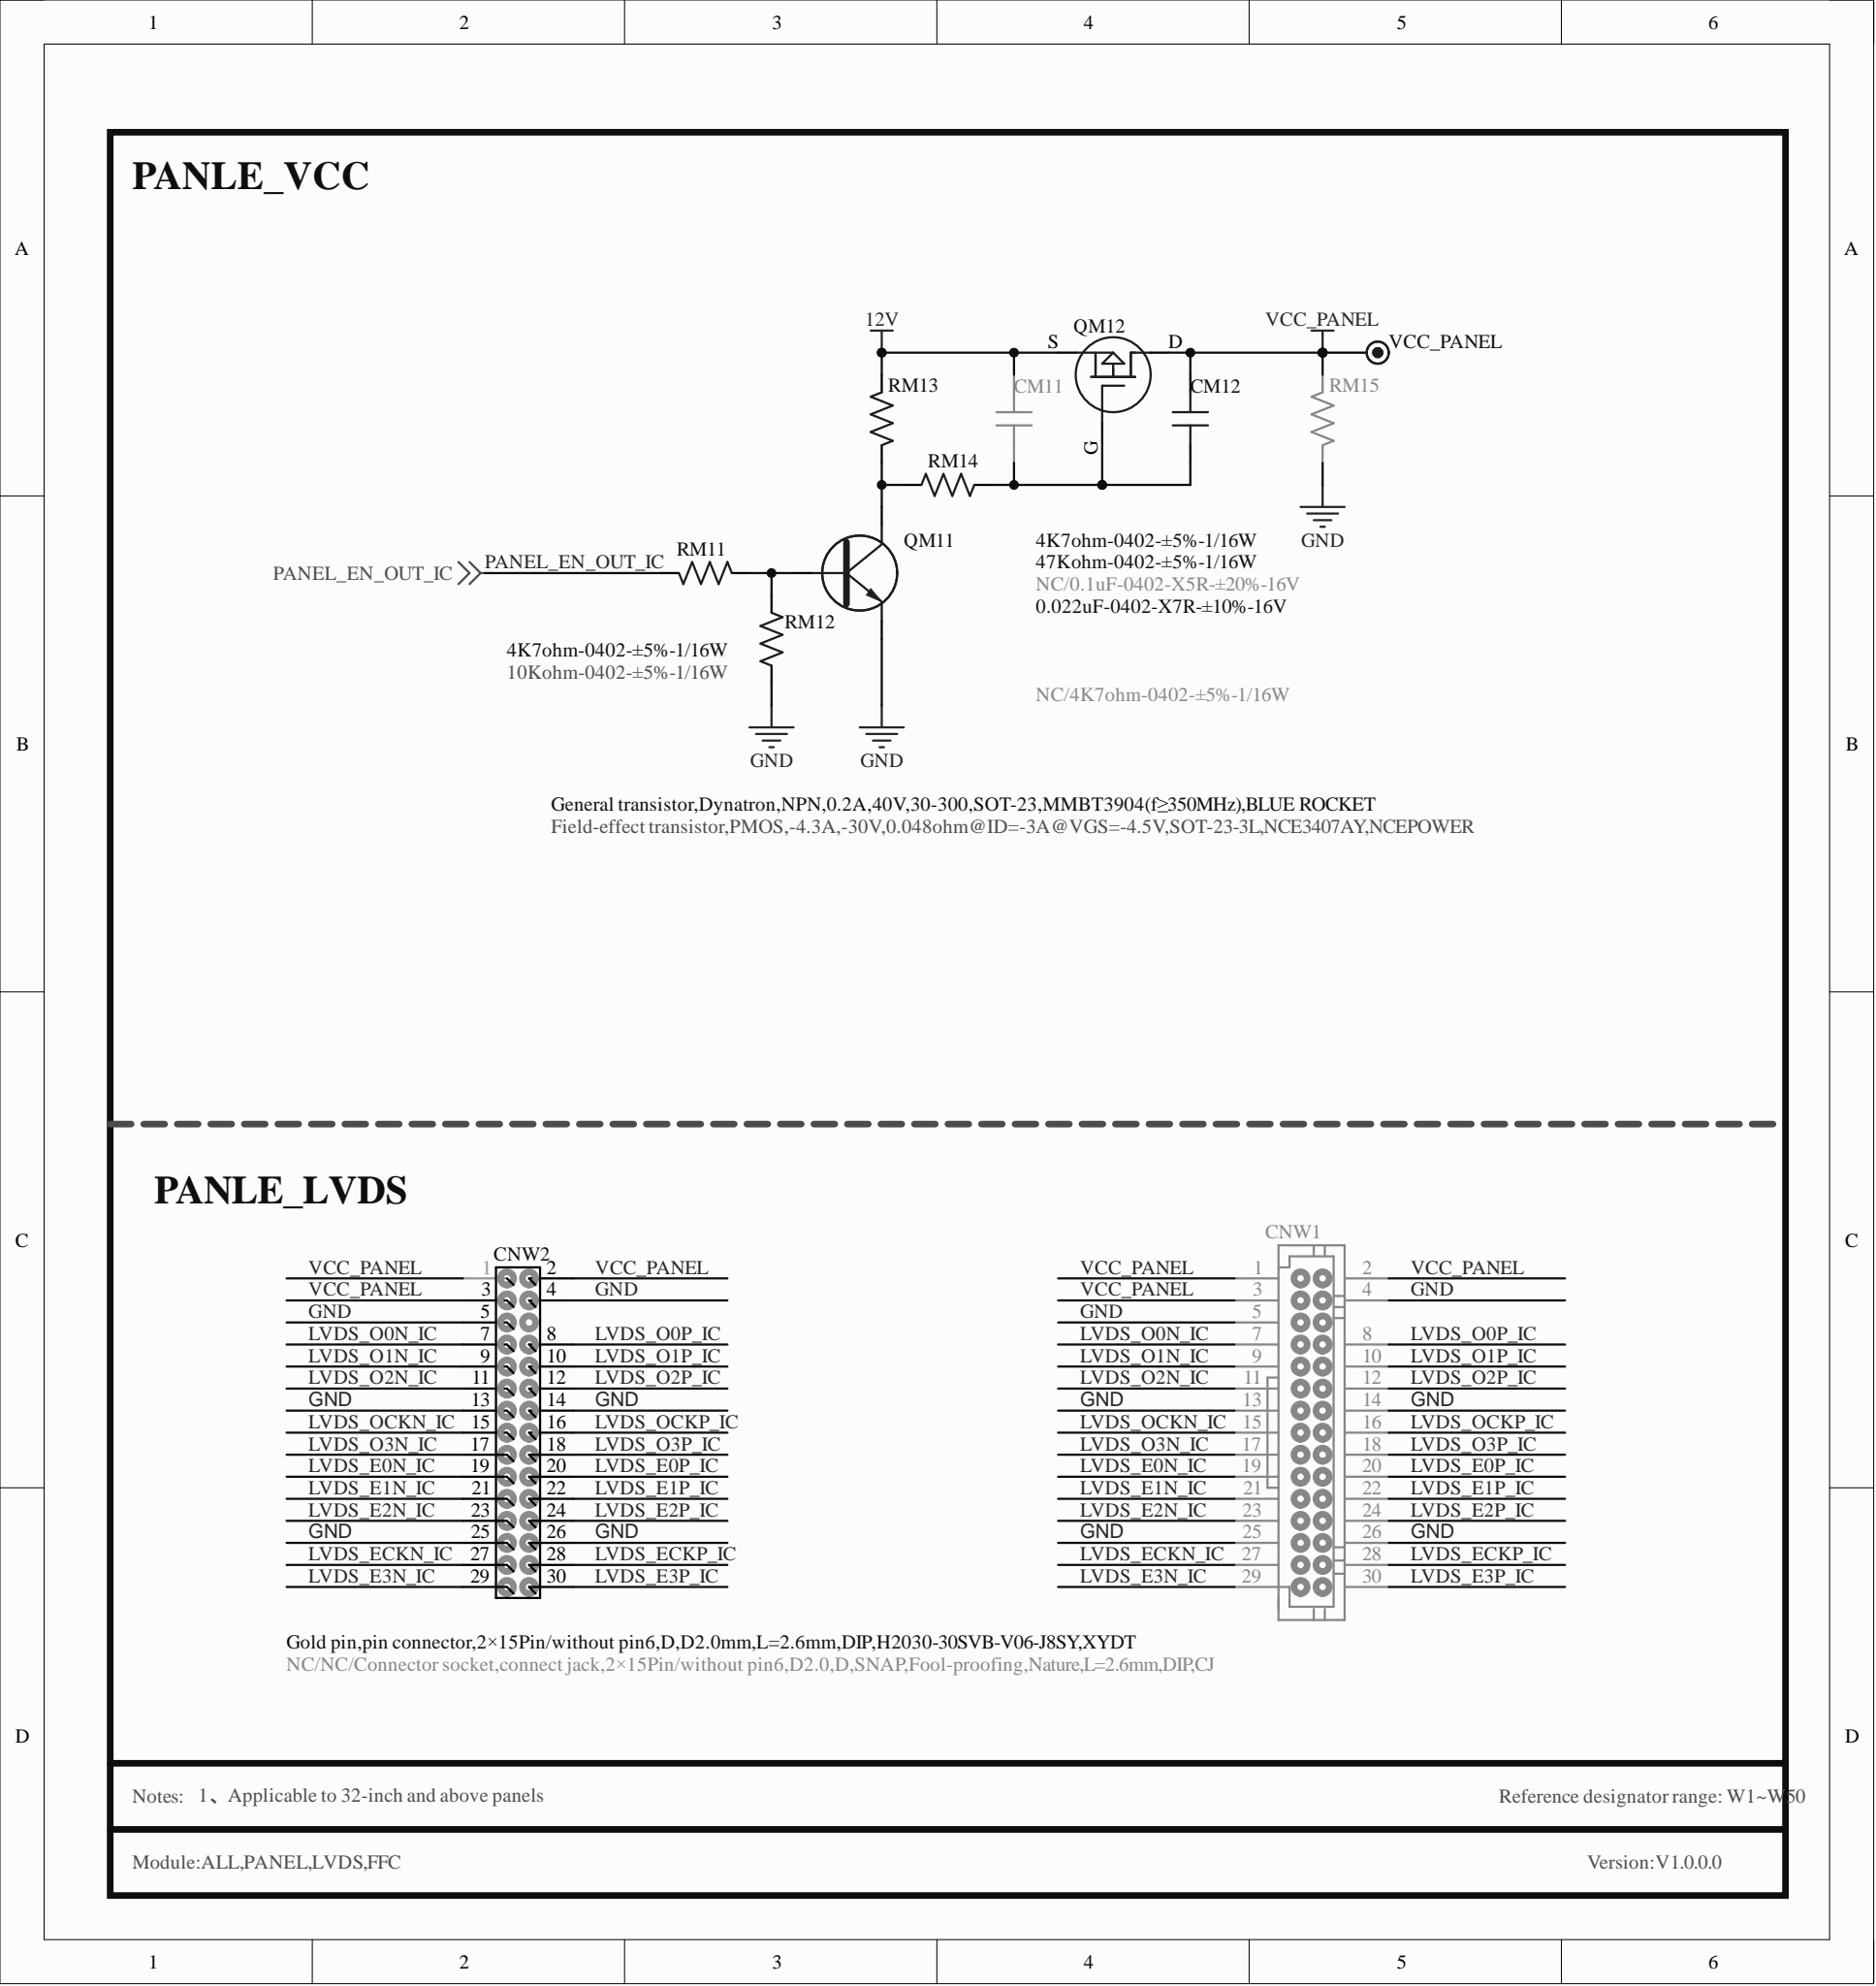Circuit board | Altium Designer | 578 parts | 300 nets | one sheet of the schematic
Parts on this sheet (reference | value | footprint):
CM11 | NC/0.1uF-0402-X5R-±20%-16V | C0402
CM12 | 0.022uF-0402-X7R-±10%-16V | C0402
CNW1 | NC/NC/Connector socket,connect jack,2×15Pin/without pin6,D2.0,D,SNAP,Fool-proofing,Nature,L=2.6mm,DIP,CJ | SIP2*15/2.0D-11
CNW2 | Gold pin,pin connector,2×15Pin/without pin6,D,D2.0mm,L=2.6mm,DIP,H2030-30SVB-V06-J8SY,XYDT | SIP2*15/2.0D-2
QM11 | General transistor,Dynatron,NPN,0.2A,40V,30-300,SOT-23,MMBT3904(f=350MHz),BLUE ROCKET | SOT-23
QM12 | Field-effect transistor,PMOS,-4.3A,-30V,0.048ohm@ID=-3A@VGS=-4.5V,SOT-23-3L,NCE3407AY,NCEPOWER | SOT-23-1
RM11 | 4K7ohm-0402-±5%-1/16W | R0402
RM12 | 10Kohm-0402-±5%-1/16W | R0402
RM13 | 4K7ohm-0402-±5%-1/16W | R0402
RM14 | 47Kohm-0402-±5%-1/16W | R0402
RM15 | NC/4K7ohm-0402-±5%-1/16W | R0402
VCC_PANEL | TEST | TP
Nets of these parts (net: part-pin ...):
VCC_PANEL: CM12-1 QM12-D RM15-1 VCC_PANEL-1 CNW1-1 CNW1-2 CNW1-3 CNW2-1 CNW2-2 CNW2-3
PANEL_EN_OUT_IC: RM11-1
NetQM11_C: QM11-C RM13-2 RM14-1
NetQM11_B: QM11-B RM11-2 RM12-1
NetCM11_1: CM11-1 CM12-2 QM12-G RM14-2
LVDS_OCKP_IC: CNW1-16 CNW2-16
LVDS_OCKN_IC: CNW1-15 CNW2-15
LVDS_O3P_IC: CNW1-18 CNW2-18
LVDS_O3N_IC: CNW1-17 CNW2-17
LVDS_O2P_IC: CNW1-12 CNW2-12
LVDS_O2N_IC: CNW1-11 CNW2-11
LVDS_O1P_IC: CNW1-10 CNW2-10
LVDS_O1N_IC: CNW1-9 CNW2-9
LVDS_O0P_IC: CNW1-8 CNW2-8
LVDS_O0N_IC: CNW1-7 CNW2-7
LVDS_ECKP_IC: CNW1-28 CNW2-28
LVDS_ECKN_IC: CNW1-27 CNW2-27
LVDS_E3P_IC: CNW1-30 CNW2-30
LVDS_E3N_IC: CNW1-29 CNW2-29
LVDS_E2P_IC: CNW1-24 CNW2-24
LVDS_E2N_IC: CNW1-23 CNW2-23
LVDS_E1P_IC: CNW1-22 CNW2-22
LVDS_E1N_IC: CNW1-21 CNW2-21
LVDS_E0P_IC: CNW1-20 CNW2-20
LVDS_E0N_IC: CNW1-19 CNW2-19
GND: QM11-E RM12-2 RM15-2 CNW1-4 CNW1-5 CNW1-13 CNW1-14 CNW1-25 CNW1-26 CNW2-4 CNW2-5 CNW2-13 CNW2-14 CNW2-25 CNW2-26
12V: CM11-2 QM12-S RM13-1